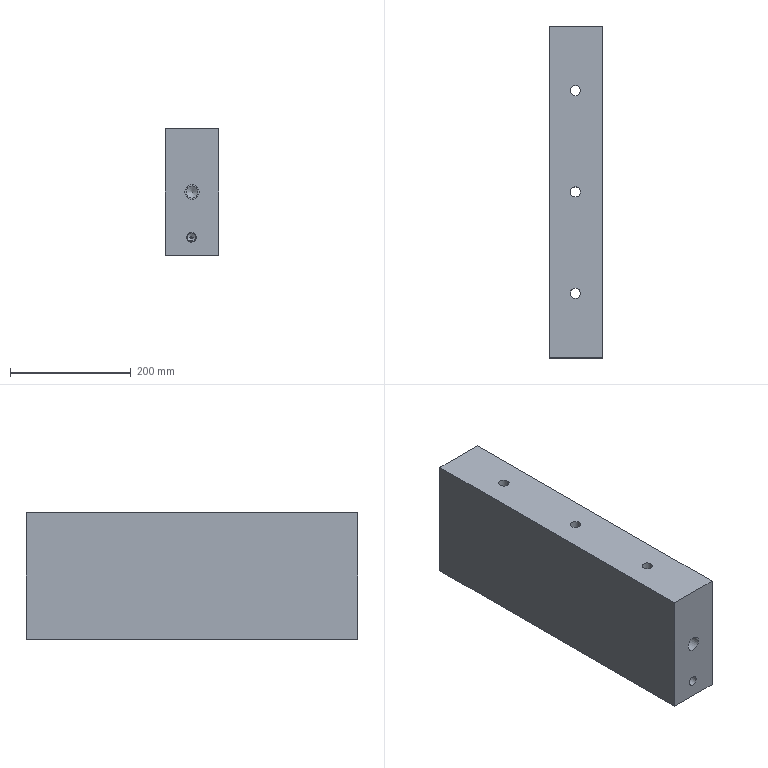Part | STEP file | 车灯-后视镜_id522_x_t | 1 solid | 29 faces | box 88 x 550 x 210 mm | volume 9957650 mm3 | cylinder 13 | plane 11 | cone 5 | commonest cylinder face diameters 17 x3 10.2 x2 12 x2 20 x2 24 x2 14.2 x1
STEP:
#1=CARTESIAN_POINT('',(210.1,232.,-345.5));
#2=VERTEX_POINT('',#1);
#3=CARTESIAN_POINT('',(205.,232.,-345.5));
#4=DIRECTION('',(0.,0.,1.));
#5=DIRECTION('',(1.,0.,0.));
#6=AXIS2_PLACEMENT_3D('',#3,#4,#5);
#7=CIRCLE('',#6,5.1);
#8=EDGE_CURVE('',#2,#2,#7,.T.);
#9=ORIENTED_EDGE('',*,*,#8,.T.);
#10=EDGE_LOOP('',(#9));
#11=FACE_BOUND('',#10,.T.);
#12=CARTESIAN_POINT('',(205.,238.,-345.5));
#13=VERTEX_POINT('',#12);
#14=CARTESIAN_POINT('',(205.,232.,-345.5));
#15=DIRECTION('',(0.,0.,-1.));
#16=DIRECTION('',(0.,1.,0.));
#17=AXIS2_PLACEMENT_3D('',#14,#15,#16);
#18=CIRCLE('',#17,6.);
#19=EDGE_CURVE('',#13,#13,#18,.T.);
#20=ORIENTED_EDGE('',*,*,#19,.T.);
#21=EDGE_LOOP('',(#20));
#22=FACE_BOUND('',#21,.T.);
#23=CARTESIAN_POINT('',(205.,232.,-345.5));
#24=DIRECTION('',(0.,0.,1.));
#25=DIRECTION('',(0.,-1.,0.));
#26=AXIS2_PLACEMENT_3D('',#23,#24,#25);
#27=PLANE('',#26);
#28=ADVANCED_FACE('',(#11,#22),#27,.F.);
#29=ORIENTED_EDGE('',*,*,#19,.F.);
#30=EDGE_LOOP('',(#29));
#31=FACE_BOUND('',#30,.T.);
#32=CARTESIAN_POINT('',(211.,232.,-370.5));
#33=VERTEX_POINT('',#32);
#34=CARTESIAN_POINT('',(205.,232.,-370.5));
#35=DIRECTION('',(0.,0.,-1.));
#36=DIRECTION('',(1.,0.,0.));
#37=AXIS2_PLACEMENT_3D('',#34,#35,#36);
#38=CIRCLE('',#37,6.);
#39=EDGE_CURVE('',#33,#33,#38,.T.);
#40=ORIENTED_EDGE('',*,*,#39,.T.);
#41=EDGE_LOOP('',(#40));
#42=FACE_BOUND('',#41,.T.);
#43=CARTESIAN_POINT('',(205.,232.,-370.5));
#44=DIRECTION('',(0.,0.,1.));
#45=DIRECTION('',(0.,-1.,0.));
#46=AXIS2_PLACEMENT_3D('',#43,#44,#45);
#47=CYLINDRICAL_SURFACE('',#46,6.);
#48=ADVANCED_FACE('',(#31,#42),#47,.F.);
#49=ORIENTED_EDGE('',*,*,#8,.F.);
#50=EDGE_LOOP('',(#49));
#51=FACE_BOUND('',#50,.T.);
#52=CARTESIAN_POINT('',(205.,237.1,-340.5));
#53=VERTEX_POINT('',#52);
#54=CARTESIAN_POINT('',(205.,232.,-340.5));
#55=DIRECTION('',(0.,0.,-1.));
#56=DIRECTION('',(0.,1.,0.));
#57=AXIS2_PLACEMENT_3D('',#54,#55,#56);
#58=CIRCLE('',#57,5.1);
#59=EDGE_CURVE('',#53,#53,#58,.T.);
#60=ORIENTED_EDGE('',*,*,#59,.F.);
#61=EDGE_LOOP('',(#60));
#62=FACE_BOUND('',#61,.T.);
#63=CARTESIAN_POINT('',(205.,232.,-370.5));
#64=DIRECTION('',(0.,0.,1.));
#65=DIRECTION('',(0.,-1.,0.));
#66=AXIS2_PLACEMENT_3D('',#63,#64,#65);
#67=CYLINDRICAL_SURFACE('',#66,5.1);
#68=ADVANCED_FACE('',(#51,#62),#67,.F.);
#69=ORIENTED_EDGE('',*,*,#59,.T.);
#70=EDGE_LOOP('',(#69));
#71=FACE_BOUND('',#70,.T.);
#72=CARTESIAN_POINT('',(205.,232.,-337.556));
#73=VERTEX_POINT('',#72);
#74=VERTEX_LOOP('',#73);
#75=FACE_BOUND('',#74,.T.);
#76=CARTESIAN_POINT('',(205.,232.,-337.556));
#77=DIRECTION('',(0.,0.,-1.));
#78=DIRECTION('',(0.,1.,0.));
#79=AXIS2_PLACEMENT_3D('',#76,#77,#78);
#80=CONICAL_SURFACE('',#79,0.,60.);
#81=ADVANCED_FACE('',(#71,#75),#80,.F.);
#82=CARTESIAN_POINT('',(250.,-275.,-370.5));
#83=VERTEX_POINT('',#82);
#84=CARTESIAN_POINT('',(162.,-275.,-370.5));
#85=VERTEX_POINT('',#84);
#86=CARTESIAN_POINT('',(210.,-275.,-370.5));
#87=DIRECTION('',(-1.,0.,0.));
#88=VECTOR('',#87,1.);
#89=LINE('',#86,#88);
#90=EDGE_CURVE('',#83,#85,#89,.T.);
#91=ORIENTED_EDGE('',*,*,#90,.T.);
#92=CARTESIAN_POINT('',(162.,275.,-370.5));
#93=VERTEX_POINT('',#92);
#94=CARTESIAN_POINT('',(162.,0.,-370.5));
#95=DIRECTION('',(0.,-1.,0.));
#96=VECTOR('',#95,1.);
#97=LINE('',#94,#96);
#98=EDGE_CURVE('',#93,#85,#97,.T.);
#99=ORIENTED_EDGE('',*,*,#98,.F.);
#100=CARTESIAN_POINT('',(250.,275.,-370.5));
#101=VERTEX_POINT('',#100);
#102=CARTESIAN_POINT('',(210.,275.,-370.5));
#103=DIRECTION('',(1.,0.,0.));
#104=VECTOR('',#103,1.);
#105=LINE('',#102,#104);
#106=EDGE_CURVE('',#93,#101,#105,.T.);
#107=ORIENTED_EDGE('',*,*,#106,.T.);
#108=CARTESIAN_POINT('',(250.,0.,-370.5));
#109=DIRECTION('',(0.,1.,0.));
#110=VECTOR('',#109,1.);
#111=LINE('',#108,#110);
#112=EDGE_CURVE('',#83,#101,#111,.T.);
#113=ORIENTED_EDGE('',*,*,#112,.F.);
#114=EDGE_LOOP('',(#91,#99,#107,#113));
#115=FACE_BOUND('',#114,.T.);
#116=ORIENTED_EDGE('',*,*,#39,.F.);
#117=EDGE_LOOP('',(#116));
#118=FACE_BOUND('',#117,.T.);
#119=CARTESIAN_POINT('',(213.5,168.,-370.5));
#120=VERTEX_POINT('',#119);
#121=CARTESIAN_POINT('',(205.,168.,-370.5));
#122=DIRECTION('',(0.,0.,-1.));
#123=DIRECTION('',(1.,0.,0.));
#124=AXIS2_PLACEMENT_3D('',#121,#122,#123);
#125=CIRCLE('',#124,8.5);
#126=EDGE_CURVE('',#120,#120,#125,.T.);
#127=ORIENTED_EDGE('',*,*,#126,.F.);
#128=EDGE_LOOP('',(#127));
#129=FACE_BOUND('',#128,.T.);
#130=CARTESIAN_POINT('',(213.5,0.,-370.5));
#131=VERTEX_POINT('',#130);
#132=CARTESIAN_POINT('',(205.,0.,-370.5));
#133=DIRECTION('',(0.,0.,-1.));
#134=DIRECTION('',(1.,0.,0.));
#135=AXIS2_PLACEMENT_3D('',#132,#133,#134);
#136=CIRCLE('',#135,8.5);
#137=EDGE_CURVE('',#131,#131,#136,.T.);
#138=ORIENTED_EDGE('',*,*,#137,.F.);
#139=EDGE_LOOP('',(#138));
#140=FACE_BOUND('',#139,.T.);
#141=CARTESIAN_POINT('',(213.5,-168.,-370.5));
#142=VERTEX_POINT('',#141);
#143=CARTESIAN_POINT('',(205.,-168.,-370.5));
#144=DIRECTION('',(0.,0.,-1.));
#145=DIRECTION('',(1.,0.,0.));
#146=AXIS2_PLACEMENT_3D('',#143,#144,#145);
#147=CIRCLE('',#146,8.5);
#148=EDGE_CURVE('',#142,#142,#147,.T.);
#149=ORIENTED_EDGE('',*,*,#148,.F.);
#150=EDGE_LOOP('',(#149));
#151=FACE_BOUND('',#150,.T.);
#152=CARTESIAN_POINT('',(211.,-232.,-370.5));
#153=VERTEX_POINT('',#152);
#154=CARTESIAN_POINT('',(205.,-232.,-370.5));
#155=DIRECTION('',(0.,0.,-1.));
#156=DIRECTION('',(1.,0.,0.));
#157=AXIS2_PLACEMENT_3D('',#154,#155,#156);
#158=CIRCLE('',#157,6.);
#159=EDGE_CURVE('',#153,#153,#158,.T.);
#160=ORIENTED_EDGE('',*,*,#159,.F.);
#161=EDGE_LOOP('',(#160));
#162=FACE_BOUND('',#161,.T.);
#163=CARTESIAN_POINT('',(210.,307.,-370.5));
#164=DIRECTION('',(0.,0.,1.));
#165=DIRECTION('',(1.,0.,0.));
#166=AXIS2_PLACEMENT_3D('',#163,#164,#165);
#167=PLANE('',#166);
#168=ADVANCED_FACE('',(#115,#118,#129,#140,#151,#162),#167,.F.);
#169=CARTESIAN_POINT('',(206.755,-236.788,-340.5));
#170=VERTEX_POINT('',#169);
#171=CARTESIAN_POINT('',(203.245,-236.788,-340.5));
#172=VERTEX_POINT('',#171);
#173=CARTESIAN_POINT('',(205.,-232.,-340.5));
#174=DIRECTION('',(0.,0.,1.));
#175=DIRECTION('',(0.,-1.,0.));
#176=AXIS2_PLACEMENT_3D('',#173,#174,#175);
#177=CIRCLE('',#176,5.1);
#178=EDGE_CURVE('',#170,#172,#177,.T.);
#179=ORIENTED_EDGE('',*,*,#178,.F.);
#180=CARTESIAN_POINT('',(206.755,-236.788,-340.5));
#181=CARTESIAN_POINT('',(206.473,-236.619,-340.352));
#182=CARTESIAN_POINT('',(206.182,-236.451,-340.21));
#183=CARTESIAN_POINT('',(205.87,-236.311,-340.094));
#184=CARTESIAN_POINT('',(205.713,-236.24,-340.037));
#185=CARTESIAN_POINT('',(205.549,-236.176,-339.985));
#186=CARTESIAN_POINT('',(205.376,-236.133,-339.952));
#187=CARTESIAN_POINT('',(205.244,-236.101,-339.926));
#188=CARTESIAN_POINT('',(205.104,-236.083,-339.912));
#189=CARTESIAN_POINT('',(204.967,-236.086,-339.915));
#190=CARTESIAN_POINT('',(204.829,-236.089,-339.917));
#191=CARTESIAN_POINT('',(204.691,-236.114,-339.936));
#192=CARTESIAN_POINT('',(204.561,-236.15,-339.965));
#193=CARTESIAN_POINT('',(204.217,-236.246,-340.041));
#194=CARTESIAN_POINT('',(203.909,-236.41,-340.175));
#195=CARTESIAN_POINT('',(203.615,-236.573,-340.314));
#196=CARTESIAN_POINT('',(203.49,-236.643,-340.374));
#197=CARTESIAN_POINT('',(203.366,-236.715,-340.436));
#198=CARTESIAN_POINT('',(203.245,-236.788,-340.5));
#199=B_SPLINE_CURVE_WITH_KNOTS('',3,(#180,#181,#182,#183,#184,#185,#186,#187,#188,#189,#190,#191,#192,#193,#194,#195,#196,#197,#198),.UNSPECIFIED.,.F.,.F.,(4,3,3,3,3,3,4),(0.,0.2689,0.404,0.507,0.6099,0.8838,1.),.UNSPECIFIED.);
#200=EDGE_CURVE('',#170,#172,#199,.T.);
#201=ORIENTED_EDGE('',*,*,#200,.T.);
#202=EDGE_LOOP('',(#179,#201));
#203=FACE_BOUND('',#202,.T.);
#204=CARTESIAN_POINT('',(205.,-232.,-337.556));
#205=VERTEX_POINT('',#204);
#206=VERTEX_LOOP('',#205);
#207=FACE_BOUND('',#206,.T.);
#208=CARTESIAN_POINT('',(205.,-232.,-337.556));
#209=DIRECTION('',(0.,0.,-1.));
#210=DIRECTION('',(0.,-1.,0.));
#211=AXIS2_PLACEMENT_3D('',#208,#209,#210);
#212=CONICAL_SURFACE('',#211,0.,60.);
#213=ADVANCED_FACE('',(#203,#207),#212,.F.);
#214=CARTESIAN_POINT('',(210.1,-232.,-345.5));
#215=VERTEX_POINT('',#214);
#216=CARTESIAN_POINT('',(205.,-232.,-345.5));
#217=DIRECTION('',(0.,0.,-1.));
#218=DIRECTION('',(1.,0.,0.));
#219=AXIS2_PLACEMENT_3D('',#216,#217,#218);
#220=CIRCLE('',#219,5.1);
#221=EDGE_CURVE('',#215,#215,#220,.T.);
#222=ORIENTED_EDGE('',*,*,#221,.T.);
#223=EDGE_LOOP('',(#222));
#224=FACE_BOUND('',#223,.T.);
#225=ORIENTED_EDGE('',*,*,#178,.T.);
#226=CARTESIAN_POINT('',(203.245,-236.788,-340.5));
#227=CARTESIAN_POINT('',(203.245,-236.788,-340.797));
#228=CARTESIAN_POINT('',(203.293,-236.807,-341.098));
#229=CARTESIAN_POINT('',(203.386,-236.838,-341.378));
#230=CARTESIAN_POINT('',(203.479,-236.869,-341.658));
#231=CARTESIAN_POINT('',(203.621,-236.914,-341.927));
#232=CARTESIAN_POINT('',(203.808,-236.959,-342.153));
#233=CARTESIAN_POINT('',(203.933,-236.989,-342.306));
#234=CARTESIAN_POINT('',(204.082,-237.02,-342.442));
#235=CARTESIAN_POINT('',(204.249,-237.044,-342.548));
#236=CARTESIAN_POINT('',(204.383,-237.064,-342.632));
#237=CARTESIAN_POINT('',(204.532,-237.081,-342.698));
#238=CARTESIAN_POINT('',(204.687,-237.09,-342.736));
#239=CARTESIAN_POINT('',(204.843,-237.1,-342.774));
#240=CARTESIAN_POINT('',(205.009,-237.102,-342.783));
#241=CARTESIAN_POINT('',(205.168,-237.097,-342.763));
#242=CARTESIAN_POINT('',(205.31,-237.093,-342.744));
#243=CARTESIAN_POINT('',(205.45,-237.082,-342.702));
#244=CARTESIAN_POINT('',(205.579,-237.067,-342.642));
#245=CARTESIAN_POINT('',(205.747,-237.048,-342.563));
#246=CARTESIAN_POINT('',(205.9,-237.022,-342.453));
#247=CARTESIAN_POINT('',(206.033,-236.994,-342.326));
#248=CARTESIAN_POINT('',(206.208,-236.958,-342.157));
#249=CARTESIAN_POINT('',(206.352,-236.919,-341.955));
#250=CARTESIAN_POINT('',(206.463,-236.886,-341.738));
#251=CARTESIAN_POINT('',(206.576,-236.852,-341.517));
#252=CARTESIAN_POINT('',(206.657,-236.823,-341.276));
#253=CARTESIAN_POINT('',(206.705,-236.807,-341.031));
#254=CARTESIAN_POINT('',(206.738,-236.795,-340.857));
#255=CARTESIAN_POINT('',(206.755,-236.788,-340.678));
#256=CARTESIAN_POINT('',(206.755,-236.788,-340.5));
#257=B_SPLINE_CURVE_WITH_KNOTS('',3,(#226,#227,#228,#229,#230,#231,#232,#233,#234,#235,#236,#237,#238,#239,#240,#241,#242,#243,#244,#245,#246,#247,#248,#249,#250,#251,#252,#253,#254,#255,#256),.UNSPECIFIED.,.F.,.F.,(4,3,3,3,3,3,3,3,3,3,4),(0.,0.1408,0.2818,0.3759,0.4512,0.527,0.5944,0.6822,0.7982,0.9164,1.),.UNSPECIFIED.);
#258=EDGE_CURVE('',#172,#170,#257,.T.);
#259=ORIENTED_EDGE('',*,*,#258,.T.);
#260=EDGE_LOOP('',(#225,#259));
#261=FACE_BOUND('',#260,.T.);
#262=CARTESIAN_POINT('',(205.,-232.,-370.5));
#263=DIRECTION('',(0.,0.,1.));
#264=DIRECTION('',(0.,1.,0.));
#265=AXIS2_PLACEMENT_3D('',#262,#263,#264);
#266=CYLINDRICAL_SURFACE('',#265,5.1);
#267=ADVANCED_FACE('',(#224,#261),#266,.F.);
#268=ORIENTED_EDGE('',*,*,#221,.F.);
#269=EDGE_LOOP('',(#268));
#270=FACE_BOUND('',#269,.T.);
#271=CARTESIAN_POINT('',(205.,-238.,-345.5));
#272=VERTEX_POINT('',#271);
#273=CARTESIAN_POINT('',(205.,-232.,-345.5));
#274=DIRECTION('',(0.,0.,1.));
#275=DIRECTION('',(0.,-1.,0.));
#276=AXIS2_PLACEMENT_3D('',#273,#274,#275);
#277=CIRCLE('',#276,6.);
#278=EDGE_CURVE('',#272,#272,#277,.T.);
#279=ORIENTED_EDGE('',*,*,#278,.F.);
#280=EDGE_LOOP('',(#279));
#281=FACE_BOUND('',#280,.T.);
#282=CARTESIAN_POINT('',(205.,-232.,-345.5));
#283=DIRECTION('',(0.,0.,1.));
#284=DIRECTION('',(0.,1.,0.));
#285=AXIS2_PLACEMENT_3D('',#282,#283,#284);
#286=PLANE('',#285);
#287=ADVANCED_FACE('',(#270,#281),#286,.F.);
#288=ORIENTED_EDGE('',*,*,#278,.T.);
#289=EDGE_LOOP('',(#288));
#290=FACE_BOUND('',#289,.T.);
#291=ORIENTED_EDGE('',*,*,#159,.T.);
#292=EDGE_LOOP('',(#291));
#293=FACE_BOUND('',#292,.T.);
#294=CARTESIAN_POINT('',(205.,-232.,-370.5));
#295=DIRECTION('',(0.,0.,1.));
#296=DIRECTION('',(0.,1.,0.));
#297=AXIS2_PLACEMENT_3D('',#294,#295,#296);
#298=CYLINDRICAL_SURFACE('',#297,6.);
#299=ADVANCED_FACE('',(#290,#293),#298,.F.);
#300=ORIENTED_EDGE('',*,*,#112,.T.);
#301=CARTESIAN_POINT('',(250.,275.,-160.5));
#302=VERTEX_POINT('',#301);
#303=CARTESIAN_POINT('',(250.,275.,-220.5));
#304=DIRECTION('',(0.,0.,1.));
#305=VECTOR('',#304,1.);
#306=LINE('',#303,#305);
#307=EDGE_CURVE('',#101,#302,#306,.T.);
#308=ORIENTED_EDGE('',*,*,#307,.T.);
#309=CARTESIAN_POINT('',(250.,-275.,-160.5));
#310=VERTEX_POINT('',#309);
#311=CARTESIAN_POINT('',(250.,0.,-160.5));
#312=DIRECTION('',(0.,-1.,0.));
#313=VECTOR('',#312,1.);
#314=LINE('',#311,#313);
#315=EDGE_CURVE('',#302,#310,#314,.T.);
#316=ORIENTED_EDGE('',*,*,#315,.T.);
#317=CARTESIAN_POINT('',(250.,-275.,-315.5));
#318=DIRECTION('',(0.,0.,1.));
#319=VECTOR('',#318,1.);
#320=LINE('',#317,#319);
#321=EDGE_CURVE('',#83,#310,#320,.T.);
#322=ORIENTED_EDGE('',*,*,#321,.F.);
#323=EDGE_LOOP('',(#300,#308,#316,#322));
#324=FACE_OUTER_BOUND('',#323,.T.);
#325=CARTESIAN_POINT('',(250.,0.,-220.5));
#326=DIRECTION('',(1.,0.,0.));
#327=DIRECTION('',(0.,0.,-1.));
#328=AXIS2_PLACEMENT_3D('',#325,#326,#327);
#329=PLANE('',#328);
#330=ADVANCED_FACE('',(#324),#329,.T.);
#331=CARTESIAN_POINT('',(162.,-275.,-160.5));
#332=VERTEX_POINT('',#331);
#333=CARTESIAN_POINT('',(162.,275.,-160.5));
#334=VERTEX_POINT('',#333);
#335=CARTESIAN_POINT('',(162.,0.,-160.5));
#336=DIRECTION('',(0.,1.,0.));
#337=VECTOR('',#336,1.);
#338=LINE('',#335,#337);
#339=EDGE_CURVE('',#332,#334,#338,.T.);
#340=ORIENTED_EDGE('',*,*,#339,.T.);
#341=CARTESIAN_POINT('',(162.,275.,-100.));
#342=DIRECTION('',(0.,0.,1.));
#343=VECTOR('',#342,1.);
#344=LINE('',#341,#343);
#345=EDGE_CURVE('',#93,#334,#344,.T.);
#346=ORIENTED_EDGE('',*,*,#345,.F.);
#347=ORIENTED_EDGE('',*,*,#98,.T.);
#348=CARTESIAN_POINT('',(162.,-275.,-100.));
#349=DIRECTION('',(0.,0.,-1.));
#350=VECTOR('',#349,1.);
#351=LINE('',#348,#350);
#352=EDGE_CURVE('',#332,#85,#351,.T.);
#353=ORIENTED_EDGE('',*,*,#352,.F.);
#354=EDGE_LOOP('',(#340,#346,#347,#353));
#355=FACE_OUTER_BOUND('',#354,.T.);
#356=CARTESIAN_POINT('',(162.,0.,-100.));
#357=DIRECTION('',(1.,0.,0.));
#358=DIRECTION('',(0.,0.,-1.));
#359=AXIS2_PLACEMENT_3D('',#356,#357,#358);
#360=PLANE('',#359);
#361=ADVANCED_FACE('',(#355),#360,.F.);
#362=ORIENTED_EDGE('',*,*,#106,.F.);
#363=ORIENTED_EDGE('',*,*,#345,.T.);
#364=CARTESIAN_POINT('',(25.,275.,-160.5));
#365=DIRECTION('',(1.,0.,0.));
#366=VECTOR('',#365,1.);
#367=LINE('',#364,#366);
#368=EDGE_CURVE('',#334,#302,#367,.T.);
#369=ORIENTED_EDGE('',*,*,#368,.T.);
#370=ORIENTED_EDGE('',*,*,#307,.F.);
#371=EDGE_LOOP('',(#362,#363,#369,#370));
#372=FACE_BOUND('',#371,.T.);
#373=CARTESIAN_POINT('',(206.,275.,-253.5));
#374=VERTEX_POINT('',#373);
#375=CARTESIAN_POINT('',(206.,275.,-265.5));
#376=DIRECTION('',(0.,-1.,0.));
#377=DIRECTION('',(0.,0.,1.));
#378=AXIS2_PLACEMENT_3D('',#375,#376,#377);
#379=CIRCLE('',#378,12.);
#380=EDGE_CURVE('',#374,#374,#379,.T.);
#381=ORIENTED_EDGE('',*,*,#380,.T.);
#382=EDGE_LOOP('',(#381));
#383=FACE_BOUND('',#382,.T.);
#384=CARTESIAN_POINT('',(25.,275.,-315.5));
#385=DIRECTION('',(0.,1.,0.));
#386=DIRECTION('',(0.,0.,1.));
#387=AXIS2_PLACEMENT_3D('',#384,#385,#386);
#388=PLANE('',#387);
#389=ADVANCED_FACE('',(#372,#383),#388,.T.);
#390=CARTESIAN_POINT('',(213.,-275.,-340.5));
#391=VERTEX_POINT('',#390);
#392=CARTESIAN_POINT('',(205.,-275.,-340.5));
#393=DIRECTION('',(0.,1.,0.));
#394=DIRECTION('',(1.,0.,0.));
#395=AXIS2_PLACEMENT_3D('',#392,#393,#394);
#396=CIRCLE('',#395,8.);
#397=EDGE_CURVE('',#391,#391,#396,.T.);
#398=ORIENTED_EDGE('',*,*,#397,.T.);
#399=EDGE_LOOP('',(#398));
#400=FACE_BOUND('',#399,.T.);
#401=CARTESIAN_POINT('',(25.,-275.,-160.5));
#402=DIRECTION('',(-1.,0.,0.));
#403=VECTOR('',#402,1.);
#404=LINE('',#401,#403);
#405=EDGE_CURVE('',#310,#332,#404,.T.);
#406=ORIENTED_EDGE('',*,*,#405,.T.);
#407=ORIENTED_EDGE('',*,*,#352,.T.);
#408=ORIENTED_EDGE('',*,*,#90,.F.);
#409=ORIENTED_EDGE('',*,*,#321,.T.);
#410=EDGE_LOOP('',(#406,#407,#408,#409));
#411=FACE_BOUND('',#410,.T.);
#412=CARTESIAN_POINT('',(206.,-275.,-277.5));
#413=VERTEX_POINT('',#412);
#414=CARTESIAN_POINT('',(206.,-275.,-265.5));
#415=DIRECTION('',(0.,-1.,0.));
#416=DIRECTION('',(0.,0.,-1.));
#417=AXIS2_PLACEMENT_3D('',#414,#415,#416);
#418=CIRCLE('',#417,12.);
#419=EDGE_CURVE('',#413,#413,#418,.T.);
#420=ORIENTED_EDGE('',*,*,#419,.F.);
#421=EDGE_LOOP('',(#420));
#422=FACE_BOUND('',#421,.T.);
#423=CARTESIAN_POINT('',(25.,-275.,-315.5));
#424=DIRECTION('',(0.,-1.,0.));
#425=DIRECTION('',(0.,0.,-1.));
#426=AXIS2_PLACEMENT_3D('',#423,#424,#425);
#427=PLANE('',#426);
#428=ADVANCED_FACE('',(#400,#411,#422),#427,.T.);
#429=ORIENTED_EDGE('',*,*,#148,.T.);
#430=EDGE_LOOP('',(#429));
#431=FACE_BOUND('',#430,.T.);
#432=CARTESIAN_POINT('',(213.5,-168.,-160.5));
#433=VERTEX_POINT('',#432);
#434=CARTESIAN_POINT('',(205.,-168.,-160.5));
#435=DIRECTION('',(0.,0.,1.));
#436=DIRECTION('',(1.,0.,0.));
#437=AXIS2_PLACEMENT_3D('',#434,#435,#436);
#438=CIRCLE('',#437,8.5);
#439=EDGE_CURVE('',#433,#433,#438,.T.);
#440=ORIENTED_EDGE('',*,*,#439,.T.);
#441=EDGE_LOOP('',(#440));
#442=FACE_BOUND('',#441,.T.);
#443=CARTESIAN_POINT('',(205.,-168.,-180.5));
#444=DIRECTION('',(0.,0.,1.));
#445=DIRECTION('',(1.,0.,0.));
#446=AXIS2_PLACEMENT_3D('',#443,#444,#445);
#447=CYLINDRICAL_SURFACE('',#446,8.5);
#448=ADVANCED_FACE('',(#431,#442),#447,.F.);
#449=ORIENTED_EDGE('',*,*,#126,.T.);
#450=EDGE_LOOP('',(#449));
#451=FACE_BOUND('',#450,.T.);
#452=CARTESIAN_POINT('',(213.5,168.,-160.5));
#453=VERTEX_POINT('',#452);
#454=CARTESIAN_POINT('',(205.,168.,-160.5));
#455=DIRECTION('',(0.,0.,-1.));
#456=DIRECTION('',(1.,0.,0.));
#457=AXIS2_PLACEMENT_3D('',#454,#455,#456);
#458=CIRCLE('',#457,8.5);
#459=EDGE_CURVE('',#453,#453,#458,.T.);
#460=ORIENTED_EDGE('',*,*,#459,.F.);
#461=EDGE_LOOP('',(#460));
#462=FACE_BOUND('',#461,.T.);
#463=CARTESIAN_POINT('',(205.,168.,-180.5));
#464=DIRECTION('',(0.,0.,1.));
#465=DIRECTION('',(1.,0.,0.));
#466=AXIS2_PLACEMENT_3D('',#463,#464,#465);
#467=CYLINDRICAL_SURFACE('',#466,8.5);
#468=ADVANCED_FACE('',(#451,#462),#467,.F.);
#469=ORIENTED_EDGE('',*,*,#339,.F.);
#470=ORIENTED_EDGE('',*,*,#405,.F.);
#471=ORIENTED_EDGE('',*,*,#315,.F.);
#472=ORIENTED_EDGE('',*,*,#368,.F.);
#473=EDGE_LOOP('',(#469,#470,#471,#472));
#474=FACE_BOUND('',#473,.T.);
#475=CARTESIAN_POINT('',(213.5,0.,-160.5));
#476=VERTEX_POINT('',#475);
#477=CARTESIAN_POINT('',(205.,0.,-160.5));
#478=DIRECTION('',(0.,0.,-1.));
#479=DIRECTION('',(1.,0.,0.));
#480=AXIS2_PLACEMENT_3D('',#477,#478,#479);
#481=CIRCLE('',#480,8.5);
#482=EDGE_CURVE('',#476,#476,#481,.T.);
#483=ORIENTED_EDGE('',*,*,#482,.T.);
#484=EDGE_LOOP('',(#483));
#485=FACE_BOUND('',#484,.T.);
#486=ORIENTED_EDGE('',*,*,#459,.T.);
#487=EDGE_LOOP('',(#486));
#488=FACE_BOUND('',#487,.T.);
#489=ORIENTED_EDGE('',*,*,#439,.F.);
#490=EDGE_LOOP('',(#489));
#491=FACE_BOUND('',#490,.T.);
#492=CARTESIAN_POINT('',(25.,0.,-160.5));
#493=DIRECTION('',(0.,0.,1.));
#494=DIRECTION('',(1.,0.,0.));
#495=AXIS2_PLACEMENT_3D('',#492,#493,#494);
#496=PLANE('',#495);
#497=ADVANCED_FACE('',(#474,#485,#488,#491),#496,.T.);
#498=ORIENTED_EDGE('',*,*,#137,.T.);
#499=EDGE_LOOP('',(#498));
#500=FACE_BOUND('',#499,.T.);
#501=ORIENTED_EDGE('',*,*,#482,.F.);
#502=EDGE_LOOP('',(#501));
#503=FACE_BOUND('',#502,.T.);
#504=CARTESIAN_POINT('',(205.,0.,-180.5));
#505=DIRECTION('',(0.,0.,1.));
#506=DIRECTION('',(1.,0.,0.));
#507=AXIS2_PLACEMENT_3D('',#504,#505,#506);
#508=CYLINDRICAL_SURFACE('',#507,8.5);
#509=ADVANCED_FACE('',(#500,#503),#508,.F.);
#510=CARTESIAN_POINT('',(206.,225.,-275.5));
#511=VERTEX_POINT('',#510);
#512=CARTESIAN_POINT('',(206.,225.,-265.5));
#513=DIRECTION('',(0.,-1.,0.));
#514=DIRECTION('',(0.,0.,-1.));
#515=AXIS2_PLACEMENT_3D('',#512,#513,#514);
#516=CIRCLE('',#515,10.);
#517=EDGE_CURVE('',#511,#511,#516,.T.);
#518=ORIENTED_EDGE('',*,*,#517,.T.);
#519=EDGE_LOOP('',(#518));
#520=FACE_BOUND('',#519,.T.);
#521=CARTESIAN_POINT('',(206.,225.,-253.5));
#522=VERTEX_POINT('',#521);
#523=CARTESIAN_POINT('',(206.,225.,-265.5));
#524=DIRECTION('',(0.,1.,0.));
#525=DIRECTION('',(0.,0.,1.));
#526=AXIS2_PLACEMENT_3D('',#523,#524,#525);
#527=CIRCLE('',#526,12.);
#528=EDGE_CURVE('',#522,#522,#527,.T.);
#529=ORIENTED_EDGE('',*,*,#528,.T.);
#530=EDGE_LOOP('',(#529));
#531=FACE_BOUND('',#530,.T.);
#532=CARTESIAN_POINT('',(206.,225.,-265.5));
#533=DIRECTION('',(0.,-1.,0.));
#534=DIRECTION('',(0.,0.,-1.));
#535=AXIS2_PLACEMENT_3D('',#532,#533,#534);
#536=PLANE('',#535);
#537=ADVANCED_FACE('',(#520,#531),#536,.F.);
#538=ORIENTED_EDGE('',*,*,#528,.F.);
#539=EDGE_LOOP('',(#538));
#540=FACE_BOUND('',#539,.T.);
#541=ORIENTED_EDGE('',*,*,#380,.F.);
#542=EDGE_LOOP('',(#541));
#543=FACE_BOUND('',#542,.T.);
#544=CARTESIAN_POINT('',(206.,275.,-265.5));
#545=DIRECTION('',(0.,-1.,0.));
#546=DIRECTION('',(0.,0.,-1.));
#547=AXIS2_PLACEMENT_3D('',#544,#545,#546);
#548=CYLINDRICAL_SURFACE('',#547,12.);
#549=ADVANCED_FACE('',(#540,#543),#548,.F.);
#550=ORIENTED_EDGE('',*,*,#517,.F.);
#551=EDGE_LOOP('',(#550));
#552=FACE_BOUND('',#551,.T.);
#553=CARTESIAN_POINT('',(206.,220.,-275.5));
#554=VERTEX_POINT('',#553);
#555=CARTESIAN_POINT('',(206.,220.,-265.5));
#556=DIRECTION('',(0.,-1.,0.));
#557=DIRECTION('',(0.,0.,-1.));
#558=AXIS2_PLACEMENT_3D('',#555,#556,#557);
#559=CIRCLE('',#558,10.);
#560=EDGE_CURVE('',#554,#554,#559,.T.);
#561=ORIENTED_EDGE('',*,*,#560,.T.);
#562=EDGE_LOOP('',(#561));
#563=FACE_BOUND('',#562,.T.);
#564=CARTESIAN_POINT('',(206.,275.,-265.5));
#565=DIRECTION('',(0.,-1.,0.));
#566=DIRECTION('',(0.,0.,-1.));
#567=AXIS2_PLACEMENT_3D('',#564,#565,#566);
#568=CYLINDRICAL_SURFACE('',#567,10.);
#569=ADVANCED_FACE('',(#552,#563),#568,.F.);
#570=ORIENTED_EDGE('',*,*,#560,.F.);
#571=EDGE_LOOP('',(#570));
#572=FACE_BOUND('',#571,.T.);
#573=CARTESIAN_POINT('',(206.,214.226,-265.5));
#574=VERTEX_POINT('',#573);
#575=VERTEX_LOOP('',#574);
#576=FACE_BOUND('',#575,.T.);
#577=CARTESIAN_POINT('',(206.,214.226,-265.5));
#578=DIRECTION('',(0.,1.,0.));
#579=DIRECTION('',(0.,0.,1.));
#580=AXIS2_PLACEMENT_3D('',#577,#578,#579);
#581=CONICAL_SURFACE('',#580,0.,60.);
#582=ADVANCED_FACE('',(#572,#576),#581,.F.);
#583=CARTESIAN_POINT('',(206.,-225.,-275.5));
#584=VERTEX_POINT('',#583);
#585=CARTESIAN_POINT('',(206.,-225.,-265.5));
#586=DIRECTION('',(0.,-1.,0.));
#587=DIRECTION('',(0.,0.,-1.));
#588=AXIS2_PLACEMENT_3D('',#585,#586,#587);
#589=CIRCLE('',#588,10.);
#590=EDGE_CURVE('',#584,#584,#589,.T.);
#591=ORIENTED_EDGE('',*,*,#590,.F.);
#592=EDGE_LOOP('',(#591));
#593=FACE_BOUND('',#592,.T.);
#594=CARTESIAN_POINT('',(206.,-225.,-253.5));
#595=VERTEX_POINT('',#594);
#596=CARTESIAN_POINT('',(206.,-225.,-265.5));
#597=DIRECTION('',(0.,1.,0.));
#598=DIRECTION('',(0.,0.,1.));
#599=AXIS2_PLACEMENT_3D('',#596,#597,#598);
#600=CIRCLE('',#599,12.);
#601=EDGE_CURVE('',#595,#595,#600,.T.);
#602=ORIENTED_EDGE('',*,*,#601,.F.);
#603=EDGE_LOOP('',(#602));
#604=FACE_BOUND('',#603,.T.);
#605=CARTESIAN_POINT('',(206.,-225.,-265.5));
#606=DIRECTION('',(0.,1.,0.));
#607=DIRECTION('',(0.,0.,-1.));
#608=AXIS2_PLACEMENT_3D('',#605,#606,#607);
#609=PLANE('',#608);
#610=ADVANCED_FACE('',(#593,#604),#609,.F.);
#611=ORIENTED_EDGE('',*,*,#601,.T.);
#612=EDGE_LOOP('',(#611));
#613=FACE_BOUND('',#612,.T.);
#614=ORIENTED_EDGE('',*,*,#419,.T.);
#615=EDGE_LOOP('',(#614));
#616=FACE_BOUND('',#615,.T.);
#617=CARTESIAN_POINT('',(206.,-275.,-265.5));
#618=DIRECTION('',(0.,1.,0.));
#619=DIRECTION('',(0.,0.,-1.));
#620=AXIS2_PLACEMENT_3D('',#617,#618,#619);
#621=CYLINDRICAL_SURFACE('',#620,12.);
#622=ADVANCED_FACE('',(#613,#616),#621,.F.);
#623=ORIENTED_EDGE('',*,*,#590,.T.);
#624=EDGE_LOOP('',(#623));
#625=FACE_BOUND('',#624,.T.);
#626=CARTESIAN_POINT('',(206.,-220.,-275.5));
#627=VERTEX_POINT('',#626);
#628=CARTESIAN_POINT('',(206.,-220.,-265.5));
#629=DIRECTION('',(0.,-1.,0.));
#630=DIRECTION('',(0.,0.,-1.));
#631=AXIS2_PLACEMENT_3D('',#628,#629,#630);
#632=CIRCLE('',#631,10.);
#633=EDGE_CURVE('',#627,#627,#632,.T.);
#634=ORIENTED_EDGE('',*,*,#633,.F.);
#635=EDGE_LOOP('',(#634));
#636=FACE_BOUND('',#635,.T.);
#637=CARTESIAN_POINT('',(206.,-275.,-265.5));
#638=DIRECTION('',(0.,1.,0.));
#639=DIRECTION('',(0.,0.,-1.));
#640=AXIS2_PLACEMENT_3D('',#637,#638,#639);
#641=CYLINDRICAL_SURFACE('',#640,10.);
#642=ADVANCED_FACE('',(#625,#636),#641,.F.);
#643=ORIENTED_EDGE('',*,*,#633,.T.);
#644=EDGE_LOOP('',(#643));
#645=FACE_BOUND('',#644,.T.);
#646=CARTESIAN_POINT('',(206.,-214.226,-265.5));
#647=VERTEX_POINT('',#646);
#648=VERTEX_LOOP('',#647);
#649=FACE_BOUND('',#648,.T.);
#650=CARTESIAN_POINT('',(206.,-214.226,-265.5));
#651=DIRECTION('',(0.,-1.,0.));
#652=DIRECTION('',(0.,0.,1.));
#653=AXIS2_PLACEMENT_3D('',#650,#651,#652);
#654=CONICAL_SURFACE('',#653,0.,60.);
#655=ADVANCED_FACE('',(#645,#649),#654,.F.);
#656=CARTESIAN_POINT('',(197.9,-240.,-340.5));
#657=VERTEX_POINT('',#656);
#658=CARTESIAN_POINT('',(205.,-240.,-340.5));
#659=DIRECTION('',(0.,-1.,0.));
#660=DIRECTION('',(-1.,0.,0.));
#661=AXIS2_PLACEMENT_3D('',#658,#659,#660);
#662=CIRCLE('',#661,7.1);
#663=EDGE_CURVE('',#657,#657,#662,.T.);
#664=ORIENTED_EDGE('',*,*,#663,.T.);
#665=EDGE_LOOP('',(#664));
#666=FACE_BOUND('',#665,.T.);
#667=ORIENTED_EDGE('',*,*,#258,.F.);
#668=ORIENTED_EDGE('',*,*,#200,.F.);
#669=EDGE_LOOP('',(#667,#668));
#670=FACE_BOUND('',#669,.T.);
#671=CARTESIAN_POINT('',(205.,-235.734,-340.5));
#672=DIRECTION('',(0.,-1.,0.));
#673=DIRECTION('',(-1.,0.,0.));
#674=AXIS2_PLACEMENT_3D('',#671,#672,#673);
#675=CONICAL_SURFACE('',#674,0.,59.);
#676=ADVANCED_FACE('',(#666,#670),#675,.F.);
#677=ORIENTED_EDGE('',*,*,#663,.F.);
#678=EDGE_LOOP('',(#677));
#679=FACE_BOUND('',#678,.T.);
#680=CARTESIAN_POINT('',(205.,-243.,-333.4));
#681=VERTEX_POINT('',#680);
#682=CARTESIAN_POINT('',(205.,-243.,-340.5));
#683=DIRECTION('',(0.,-1.,0.));
#684=DIRECTION('',(0.,0.,1.));
#685=AXIS2_PLACEMENT_3D('',#682,#683,#684);
#686=CIRCLE('',#685,7.1);
#687=EDGE_CURVE('',#681,#681,#686,.T.);
#688=ORIENTED_EDGE('',*,*,#687,.T.);
#689=EDGE_LOOP('',(#688));
#690=FACE_BOUND('',#689,.T.);
#691=CARTESIAN_POINT('',(205.,-243.,-340.5));
#692=DIRECTION('',(0.,1.,0.));
#693=DIRECTION('',(1.,0.,0.));
#694=AXIS2_PLACEMENT_3D('',#691,#692,#693);
#695=CYLINDRICAL_SURFACE('',#694,7.1);
#696=ADVANCED_FACE('',(#679,#690),#695,.F.);
#697=ORIENTED_EDGE('',*,*,#687,.F.);
#698=EDGE_LOOP('',(#697));
#699=FACE_BOUND('',#698,.T.);
#700=CARTESIAN_POINT('',(197.,-243.,-340.5));
#701=VERTEX_POINT('',#700);
#702=CARTESIAN_POINT('',(205.,-243.,-340.5));
#703=DIRECTION('',(0.,-1.,0.));
#704=DIRECTION('',(-1.,0.,0.));
#705=AXIS2_PLACEMENT_3D('',#702,#703,#704);
#706=CIRCLE('',#705,8.);
#707=EDGE_CURVE('',#701,#701,#706,.T.);
#708=ORIENTED_EDGE('',*,*,#707,.T.);
#709=EDGE_LOOP('',(#708));
#710=FACE_BOUND('',#709,.T.);
#711=CARTESIAN_POINT('',(205.,-243.,-340.5));
#712=DIRECTION('',(0.,1.,0.));
#713=DIRECTION('',(1.,0.,0.));
#714=AXIS2_PLACEMENT_3D('',#711,#712,#713);
#715=PLANE('',#714);
#716=ADVANCED_FACE('',(#699,#710),#715,.F.);
#717=ORIENTED_EDGE('',*,*,#707,.F.);
#718=EDGE_LOOP('',(#717));
#719=FACE_BOUND('',#718,.T.);
#720=ORIENTED_EDGE('',*,*,#397,.F.);
#721=EDGE_LOOP('',(#720));
#722=FACE_BOUND('',#721,.T.);
#723=CARTESIAN_POINT('',(205.,-275.,-340.5));
#724=DIRECTION('',(0.,1.,0.));
#725=DIRECTION('',(1.,0.,0.));
#726=AXIS2_PLACEMENT_3D('',#723,#724,#725);
#727=CYLINDRICAL_SURFACE('',#726,8.);
#728=ADVANCED_FACE('',(#719,#722),#727,.F.);
#729=CLOSED_SHELL('',(#28,#48,#68,#81,#168,#213,#267,#287,#299,#330,#361,#389,#428,#448,#468,#497,#509,#537,#549,#569,#582,#610,#622,#642,#655,#676,#696,#716,#728));
#730=MANIFOLD_SOLID_BREP('',#729);
#731=(LENGTH_UNIT()NAMED_UNIT(*)SI_UNIT(.MILLI.,.METRE.));
#732=UNCERTAINTY_MEASURE_WITH_UNIT(LENGTH_MEASURE(0.0508),#731,'','');
#733=(NAMED_UNIT(*)PLANE_ANGLE_UNIT()SI_UNIT($,.RADIAN.));
#734=PLANE_ANGLE_MEASURE_WITH_UNIT(PLANE_ANGLE_MEASURE(0.01745),#733);
#735=DIMENSIONAL_EXPONENTS(0.,0.,0.,0.,0.,0.,0.);
#736=(CONVERSION_BASED_UNIT('DEGREE',#734)NAMED_UNIT(#735)PLANE_ANGLE_UNIT());
#737=(NAMED_UNIT(*)SI_UNIT($,.STERADIAN.)SOLID_ANGLE_UNIT());
#738=(GEOMETRIC_REPRESENTATION_CONTEXT(3)GLOBAL_UNCERTAINTY_ASSIGNED_CONTEXT((#732))GLOBAL_UNIT_ASSIGNED_CONTEXT((#731,#736,#737))REPRESENTATION_CONTEXT('',''));
#739=ADVANCED_BREP_SHAPE_REPRESENTATION('',(#730),#738);